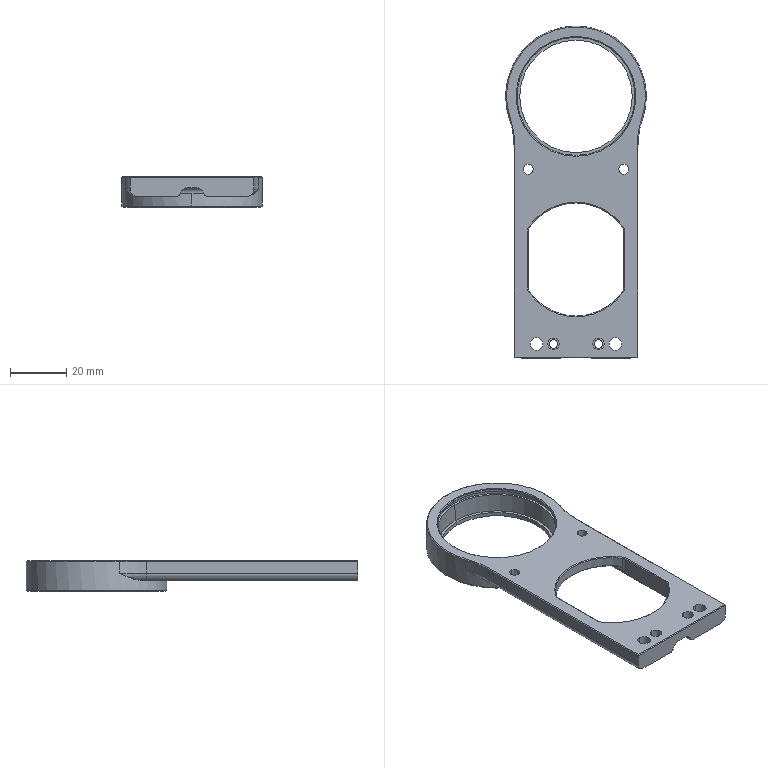NC program | NX | posted with a generic post | part box 50 x 118 x 11 mm
Lines 19 to 843 of 3723:
(ZLEVEL_PROFILE , TOOL : D10)
N36 T15 M6
N38 G54
N40 G17 G0 G90 X-64.1 Y-13.852 S9500 M3
N42 G43 Z30. H15
N44 Z1.5
N46 G94 G1 Y22.554 Z-0.408 F1000.
N48 X-63.766 Y23.898 Z-0.481
N50 X-63.084 Y25.104 Z-0.553
N52 X-62.104 Y26.084 Z-0.626
N54 X-60.898 Y26.766 Z-0.698
N56 X-59.554 Y27.1 Z-0.771
N58 X-59. Z-0.8
N60 X16.084 F3500.
N62 G3 X24.195 Y28.458 R24.9
N64 G2 X24.195 Y-28.458 R-30.1
N66 G3 X16.084 Y-27.1 R24.9
N68 G1 X-59.
N70 G2 X-64.1 Y-22. R5.1
N72 G1 Y22.
N74 G2 X-59. Y27.1 R5.1
N76 G1 X16.084 Z-0.976
N78 X17.116 Y27.121 Z-0.978
N80 X18.147 Y27.186 Z-0.981
N82 X19.174 Y27.293 Z-0.983
N84 X20.196 Y27.442 Z-0.986
N86 X21.21 Y27.634 Z-0.988
N88 X22.216 Y27.867 Z-0.991
N90 X23.212 Y28.142 Z-0.993
N92 X24.195 Y28.458 Z-0.995
N94 X25.435 Y28.856 Z-0.998
N96 X26.691 Y29.199 Z-1.002
N98 X27.96 Y29.488 Z-1.005
N100 X29.241 Y29.721 Z-1.008
N102 X30.531 Y29.899 Z-1.011
N104 X31.827 Y30.021 Z-1.014
N106 X33.127 Y30.087 Z-1.017
N108 X34.429 Y30.097 Z-1.02
N110 X35.731 Y30.05 Z-1.023
N112 X37.028 Y29.947 Z-1.026
N114 X38.321 Y29.788 Z-1.029
N116 X39.605 Y29.574 Z-1.032
N118 X40.879 Y29.304 Z-1.035
N120 X42.139 Y28.979 Z-1.038
N122 X43.385 Y28.6 Z-1.041
N124 X44.613 Y28.167 Z-1.044
N126 X45.821 Y27.682 Z-1.047
N128 X47.007 Y27.144 Z-1.05
N130 X48.169 Y26.557 Z-1.053
N132 X49.304 Y25.919 Z-1.056
N134 X50.411 Y25.233 Z-1.06
N136 X51.487 Y24.5 Z-1.063
N138 X52.53 Y23.72 Z-1.066
N140 X53.538 Y22.897 Z-1.069
N142 X54.51 Y22.031 Z-1.072
N144 X55.444 Y21.123 Z-1.075
N146 X56.337 Y20.176 Z-1.078
N148 X57.189 Y19.191 Z-1.081
N150 X57.997 Y18.17 Z-1.084
N152 X58.76 Y17.115 Z-1.087
N154 X59.477 Y16.029 Z-1.09
N156 X60.147 Y14.912 Z-1.093
N158 X60.767 Y13.767 Z-1.096
N160 X61.337 Y12.597 Z-1.099
N162 X61.857 Y11.403 Z-1.102
N164 X62.324 Y10.187 Z-1.105
N166 X62.738 Y8.953 Z-1.108
N168 X63.098 Y7.702 Z-1.111
N170 X63.404 Y6.436 Z-1.114
N172 X63.655 Y5.159 Z-1.118
N174 X63.85 Y3.871 Z-1.121
N176 X63.989 Y2.577 Z-1.124
N178 X64.073 Y1.278 Z-1.127
N180 X64.1 Y-0.024 Z-1.13
N182 X64.071 Y-1.325 Z-1.133
N184 X63.986 Y-2.623 Z-1.136
N186 X63.844 Y-3.916 Z-1.139
N188 X63.647 Y-5.202 Z-1.142
N190 X63.395 Y-6.478 Z-1.145
N192 X63.087 Y-7.742 Z-1.148
N194 X62.726 Y-8.992 Z-1.151
N196 X62.31 Y-10.225 Z-1.154
N198 X61.842 Y-11.438 Z-1.157
N200 X61.322 Y-12.631 Z-1.16
N202 X60.75 Y-13.799 Z-1.163
N204 X60.129 Y-14.942 Z-1.166
N206 X59.459 Y-16.057 Z-1.169
N208 X58.742 Y-17.143 Z-1.172
N210 X57.978 Y-18.196 Z-1.175
N212 X57.169 Y-19.215 Z-1.179
N214 X56.317 Y-20.198 Z-1.182
N216 X55.424 Y-21.143 Z-1.185
N218 X54.49 Y-22.049 Z-1.188
N220 X53.518 Y-22.914 Z-1.191
N222 X52.51 Y-23.736 Z-1.194
N224 X51.467 Y-24.514 Z-1.197
N226 X50.391 Y-25.245 Z-1.2
N228 X49.285 Y-25.93 Z-1.203
N230 X48.151 Y-26.566 Z-1.206
N232 X46.989 Y-27.153 Z-1.209
N234 X45.804 Y-27.689 Z-1.212
N236 X44.597 Y-28.173 Z-1.215
N238 X43.369 Y-28.605 Z-1.218
N240 X42.125 Y-28.983 Z-1.221
N242 X40.865 Y-29.307 Z-1.224
N244 X39.592 Y-29.576 Z-1.227
N246 X38.309 Y-29.79 Z-1.23
N248 X37.018 Y-29.948 Z-1.233
N250 X35.721 Y-30.051 Z-1.236
N252 X34.421 Y-30.097 Z-1.24
N254 X33.12 Y-30.087 Z-1.243
N256 X31.82 Y-30.021 Z-1.246
N258 X30.525 Y-29.899 Z-1.249
N260 X29.237 Y-29.721 Z-1.252
N262 X27.957 Y-29.487 Z-1.255
N264 X26.688 Y-29.198 Z-1.258
N266 X25.434 Y-28.855 Z-1.261
N268 X24.195 Y-28.458 Z-1.264
N270 X23.212 Y-28.142 Z-1.266
N272 X22.216 Y-27.867 Z-1.269
N274 X21.21 Y-27.634 Z-1.271
N276 X20.196 Y-27.442 Z-1.274
N278 X19.174 Y-27.293 Z-1.276
N280 X18.147 Y-27.186 Z-1.278
N282 X17.116 Y-27.121 Z-1.281
N284 X16.084 Y-27.1 Z-1.283
N286 X-59. Z-1.459
N288 X-59.5 Y-27.075 Z-1.46
N290 X-59.995 Y-27.002 Z-1.462
N292 X-60.48 Y-26.88 Z-1.463
N294 X-60.952 Y-26.712 Z-1.464
N296 X-61.404 Y-26.498 Z-1.465
N298 X-61.833 Y-26.24 Z-1.466
N300 X-62.235 Y-25.942 Z-1.468
N302 X-62.606 Y-25.606 Z-1.469
N304 X-62.942 Y-25.235 Z-1.47
N306 X-63.24 Y-24.833 Z-1.471
N308 X-63.498 Y-24.404 Z-1.472
N310 X-63.712 Y-23.952 Z-1.473
N312 X-63.88 Y-23.48 Z-1.475
N314 X-64.002 Y-22.995 Z-1.476
N316 X-64.075 Y-22.5 Z-1.477
N318 X-64.1 Y-22. Z-1.478
N320 Y22. Z-1.581
N322 X-64.075 Y22.5 Z-1.582
N324 X-64.002 Y22.995 Z-1.584
N326 X-63.88 Y23.48 Z-1.585
N328 X-63.712 Y23.952 Z-1.586
N330 X-63.498 Y24.404 Z-1.587
N332 X-63.24 Y24.833 Z-1.588
N334 X-62.942 Y25.235 Z-1.589
N336 X-62.606 Y25.606 Z-1.591
N338 X-62.235 Y25.942 Z-1.592
N340 X-61.833 Y26.24 Z-1.593
N342 X-61.404 Y26.498 Z-1.594
N344 X-60.952 Y26.712 Z-1.595
N346 X-60.48 Y26.88 Z-1.596
N348 X-59.995 Y27.002 Z-1.598
N350 X-59.5 Y27.075 Z-1.599
N352 X-59. Y27.1 Z-1.6
N354 X16.084 Z-1.776
N356 X17.116 Y27.121 Z-1.778
N358 X18.147 Y27.186 Z-1.781
N360 X19.174 Y27.293 Z-1.783
N362 X20.196 Y27.442 Z-1.786
N364 X21.21 Y27.634 Z-1.788
N366 X22.216 Y27.867 Z-1.791
N368 X23.212 Y28.142 Z-1.793
N370 X24.195 Y28.458 Z-1.795
N372 X25.435 Y28.856 Z-1.798
N374 X26.691 Y29.199 Z-1.802
N376 X27.96 Y29.488 Z-1.805
N378 X29.241 Y29.721 Z-1.808
N380 X30.531 Y29.899 Z-1.811
N382 X31.827 Y30.021 Z-1.814
N384 X33.127 Y30.087 Z-1.817
N386 X34.429 Y30.097 Z-1.82
N388 X35.731 Y30.05 Z-1.823
N390 X37.028 Y29.947 Z-1.826
N392 X38.321 Y29.788 Z-1.829
N394 X39.605 Y29.574 Z-1.832
N396 X40.879 Y29.304 Z-1.835
N398 X42.139 Y28.979 Z-1.838
N400 X43.385 Y28.6 Z-1.841
N402 X44.613 Y28.167 Z-1.844
N404 X45.821 Y27.682 Z-1.847
N406 X47.007 Y27.144 Z-1.85
N408 X48.169 Y26.557 Z-1.853
N410 X49.304 Y25.919 Z-1.856
N412 X50.411 Y25.233 Z-1.86
N414 X51.487 Y24.5 Z-1.863
N416 X52.53 Y23.72 Z-1.866
N418 X53.538 Y22.897 Z-1.869
N420 X54.51 Y22.031 Z-1.872
N422 X55.444 Y21.123 Z-1.875
N424 X56.337 Y20.176 Z-1.878
N426 X57.189 Y19.191 Z-1.881
N428 X57.997 Y18.17 Z-1.884
N430 X58.76 Y17.115 Z-1.887
N432 X59.477 Y16.029 Z-1.89
N434 X60.147 Y14.912 Z-1.893
N436 X60.767 Y13.767 Z-1.896
N438 X61.337 Y12.597 Z-1.899
N440 X61.857 Y11.403 Z-1.902
N442 X62.324 Y10.187 Z-1.905
N444 X62.738 Y8.953 Z-1.908
N446 X63.098 Y7.702 Z-1.911
N448 X63.404 Y6.436 Z-1.914
N450 X63.655 Y5.159 Z-1.918
N452 X63.85 Y3.871 Z-1.921
N454 X63.989 Y2.577 Z-1.924
N456 X64.073 Y1.278 Z-1.927
N458 X64.1 Y-0.024 Z-1.93
N460 X64.071 Y-1.325 Z-1.933
N462 X63.986 Y-2.623 Z-1.936
N464 X63.844 Y-3.916 Z-1.939
N466 X63.647 Y-5.202 Z-1.942
N468 X63.395 Y-6.478 Z-1.945
N470 X63.087 Y-7.742 Z-1.948
N472 X62.726 Y-8.992 Z-1.951
N474 X62.31 Y-10.225 Z-1.954
N476 X61.842 Y-11.438 Z-1.957
N478 X61.322 Y-12.631 Z-1.96
N480 X60.75 Y-13.799 Z-1.963
N482 X60.129 Y-14.942 Z-1.966
N484 X59.459 Y-16.057 Z-1.969
N486 X58.742 Y-17.143 Z-1.972
N488 X57.978 Y-18.196 Z-1.975
N490 X57.169 Y-19.215 Z-1.979
N492 X56.317 Y-20.198 Z-1.982
N494 X55.424 Y-21.143 Z-1.985
N496 X54.49 Y-22.049 Z-1.988
N498 X53.518 Y-22.914 Z-1.991
N500 X52.51 Y-23.736 Z-1.994
N502 X51.467 Y-24.514 Z-1.997
N504 X50.391 Y-25.245 Z-2.
N506 X49.285 Y-25.93 Z-2.003
N508 X48.151 Y-26.566 Z-2.006
N510 X46.989 Y-27.153 Z-2.009
N512 X45.804 Y-27.689 Z-2.012
N514 X44.597 Y-28.173 Z-2.015
N516 X43.369 Y-28.605 Z-2.018
N518 X42.125 Y-28.983 Z-2.021
N520 X40.865 Y-29.307 Z-2.024
N522 X39.592 Y-29.576 Z-2.027
N524 X38.309 Y-29.79 Z-2.03
N526 X37.018 Y-29.948 Z-2.033
N528 X35.721 Y-30.051 Z-2.036
N530 X34.421 Y-30.097 Z-2.04
N532 X33.12 Y-30.087 Z-2.043
N534 X31.82 Y-30.021 Z-2.046
N536 X30.525 Y-29.899 Z-2.049
N538 X29.237 Y-29.721 Z-2.052
N540 X27.957 Y-29.487 Z-2.055
N542 X26.688 Y-29.198 Z-2.058
N544 X25.434 Y-28.855 Z-2.061
N546 X24.195 Y-28.458 Z-2.064
N548 X23.212 Y-28.142 Z-2.066
N550 X22.216 Y-27.867 Z-2.069
N552 X21.21 Y-27.634 Z-2.071
N554 X20.196 Y-27.442 Z-2.074
N556 X19.174 Y-27.293 Z-2.076
N558 X18.147 Y-27.186 Z-2.078
N560 X17.116 Y-27.121 Z-2.081
N562 X16.084 Y-27.1 Z-2.083
N564 X-59. Z-2.259
N566 X-59.5 Y-27.075 Z-2.26
N568 X-59.995 Y-27.002 Z-2.262
N570 X-60.48 Y-26.88 Z-2.263
N572 X-60.952 Y-26.712 Z-2.264
N574 X-61.404 Y-26.498 Z-2.265
N576 X-61.833 Y-26.24 Z-2.266
N578 X-62.235 Y-25.942 Z-2.268
N580 X-62.606 Y-25.606 Z-2.269
N582 X-62.942 Y-25.235 Z-2.27
N584 X-63.24 Y-24.833 Z-2.271
N586 X-63.498 Y-24.404 Z-2.272
N588 X-63.712 Y-23.952 Z-2.273
N590 X-63.88 Y-23.48 Z-2.275
N592 X-64.002 Y-22.995 Z-2.276
N594 X-64.075 Y-22.5 Z-2.277
N596 X-64.1 Y-22. Z-2.278
N598 Y22. Z-2.381
N600 X-64.075 Y22.5 Z-2.382
N602 X-64.002 Y22.995 Z-2.384
N604 X-63.88 Y23.48 Z-2.385
N606 X-63.712 Y23.952 Z-2.386
N608 X-63.498 Y24.404 Z-2.387
N610 X-63.24 Y24.833 Z-2.388
N612 X-62.942 Y25.235 Z-2.389
N614 X-62.606 Y25.606 Z-2.391
N616 X-62.235 Y25.942 Z-2.392
N618 X-61.833 Y26.24 Z-2.393
N620 X-61.404 Y26.498 Z-2.394
N622 X-60.952 Y26.712 Z-2.395
N624 X-60.48 Y26.88 Z-2.396
N626 X-59.995 Y27.002 Z-2.398
N628 X-59.5 Y27.075 Z-2.399
N630 X-59. Y27.1 Z-2.4
N632 X16.084 Z-2.583
N634 X17.116 Y27.121 Z-2.586
N636 X18.147 Y27.186 Z-2.588
N638 X19.174 Y27.293 Z-2.591
N640 X20.196 Y27.442 Z-2.593
N642 X21.21 Y27.634 Z-2.596
N644 X22.216 Y27.867 Z-2.599
N646 X23.212 Y28.142 Z-2.601
N648 X24.195 Y28.458 Z-2.604
N650 X25.435 Y28.856 Z-2.607
N652 X26.691 Y29.199 Z-2.61
N654 X27.96 Y29.488 Z-2.613
N656 X29.241 Y29.721 Z-2.616
N658 X30.531 Y29.899 Z-2.619
N660 X31.827 Y30.021 Z-2.623
N662 X33.127 Y30.087 Z-2.626
N664 X34.429 Y30.097 Z-2.629
N666 X35.731 Y30.05 Z-2.632
N668 X37.028 Y29.947 Z-2.635
N670 X38.321 Y29.788 Z-2.639
N672 X39.605 Y29.574 Z-2.642
N674 X40.879 Y29.304 Z-2.645
N676 X42.139 Y28.979 Z-2.648
N678 X43.385 Y28.6 Z-2.651
N680 X44.613 Y28.167 Z-2.654
N682 X45.821 Y27.682 Z-2.658
N684 X47.007 Y27.144 Z-2.661
N686 X48.169 Y26.557 Z-2.664
N688 X49.304 Y25.919 Z-2.667
N690 X50.411 Y25.233 Z-2.67
N692 X51.487 Y24.5 Z-2.674
N694 X52.53 Y23.72 Z-2.677
N696 X53.538 Y22.897 Z-2.68
N698 X54.51 Y22.031 Z-2.683
N700 X55.444 Y21.123 Z-2.686
N702 X56.337 Y20.176 Z-2.689
N704 X57.189 Y19.191 Z-2.693
N706 X57.997 Y18.17 Z-2.696
N708 X58.76 Y17.115 Z-2.699
N710 X59.477 Y16.029 Z-2.702
N712 X60.147 Y14.912 Z-2.705
N714 X60.767 Y13.767 Z-2.708
N716 X61.337 Y12.597 Z-2.712
N718 X61.857 Y11.403 Z-2.715
N720 X62.324 Y10.187 Z-2.718
N722 X62.738 Y8.953 Z-2.721
N724 X63.098 Y7.702 Z-2.724
N726 X63.404 Y6.436 Z-2.728
N728 X63.655 Y5.159 Z-2.731
N730 X63.85 Y3.871 Z-2.734
N732 X63.989 Y2.577 Z-2.737
N734 X64.073 Y1.278 Z-2.74
N736 X64.1 Y-0.024 Z-2.743
N738 X64.071 Y-1.325 Z-2.747
N740 X63.986 Y-2.623 Z-2.75
N742 X63.844 Y-3.916 Z-2.753
N744 X63.647 Y-5.202 Z-2.756
N746 X63.395 Y-6.478 Z-2.759
N748 X63.087 Y-7.742 Z-2.763
N750 X62.726 Y-8.992 Z-2.766
N752 X62.31 Y-10.225 Z-2.769
N754 X61.842 Y-11.438 Z-2.772
N756 X61.322 Y-12.631 Z-2.775
N758 X60.75 Y-13.799 Z-2.778
N760 X60.129 Y-14.942 Z-2.782
N762 X59.459 Y-16.057 Z-2.785
N764 X58.742 Y-17.143 Z-2.788
N766 X57.978 Y-18.196 Z-2.791
N768 X57.169 Y-19.215 Z-2.794
N770 X56.317 Y-20.198 Z-2.797
N772 X55.424 Y-21.143 Z-2.801
N774 X54.49 Y-22.049 Z-2.804
N776 X53.518 Y-22.914 Z-2.807
N778 X52.51 Y-23.736 Z-2.81
N780 X51.467 Y-24.514 Z-2.813
N782 X50.391 Y-25.245 Z-2.817
N784 X49.285 Y-25.93 Z-2.82
N786 X48.151 Y-26.566 Z-2.823
N788 X46.989 Y-27.153 Z-2.826
N790 X45.804 Y-27.689 Z-2.829
N792 X44.597 Y-28.173 Z-2.832
N794 X43.369 Y-28.605 Z-2.836
N796 X42.125 Y-28.983 Z-2.839
N798 X40.865 Y-29.307 Z-2.842
N800 X39.592 Y-29.576 Z-2.845
N802 X38.309 Y-29.79 Z-2.848
N804 X37.018 Y-29.948 Z-2.851
N806 X35.721 Y-30.051 Z-2.855
N808 X34.421 Y-30.097 Z-2.858
N810 X33.12 Y-30.087 Z-2.861
N812 X31.82 Y-30.021 Z-2.864
N814 X30.525 Y-29.899 Z-2.867
N816 X29.237 Y-29.721 Z-2.871
N818 X27.957 Y-29.487 Z-2.874
N820 X26.688 Y-29.198 Z-2.877
N822 X25.434 Y-28.855 Z-2.88
N824 X24.195 Y-28.458 Z-2.883
N826 X23.212 Y-28.142 Z-2.886
N828 X22.216 Y-27.867 Z-2.888
N830 X21.21 Y-27.634 Z-2.891
N832 X20.196 Y-27.442 Z-2.893
N834 X19.174 Y-27.293 Z-2.896
N836 X18.147 Y-27.186 Z-2.898
N838 X17.116 Y-27.121 Z-2.901
N840 X16.084 Y-27.1 Z-2.903
N842 X-59. Z-3.087
N844 X-59.5 Y-27.075 Z-3.088
N846 X-59.995 Y-27.002 Z-3.089
N848 X-60.48 Y-26.88 Z-3.09
N850 X-60.952 Y-26.712 Z-3.092
N852 X-61.404 Y-26.498 Z-3.093
N854 X-61.833 Y-26.24 Z-3.094
N856 X-62.235 Y-25.942 Z-3.095
N858 X-62.606 Y-25.606 Z-3.097
N860 X-62.942 Y-25.235 Z-3.098
N862 X-63.24 Y-24.833 Z-3.099
N864 X-63.498 Y-24.404 Z-3.1
N866 X-63.712 Y-23.952 Z-3.101
N868 X-63.88 Y-23.48 Z-3.103
N870 X-64.002 Y-22.995 Z-3.104
N872 X-64.075 Y-22.5 Z-3.105
N874 X-64.1 Y-22. Z-3.106
N876 Y22. Z-3.214
N878 X-64.075 Y22.5 Z-3.215
N880 X-64.002 Y22.995 Z-3.216
N882 X-63.88 Y23.48 Z-3.217
N884 X-63.712 Y23.952 Z-3.219
N886 X-63.498 Y24.404 Z-3.22
N888 X-63.24 Y24.833 Z-3.221
N890 X-62.942 Y25.235 Z-3.222
N892 X-62.606 Y25.606 Z-3.224
N894 X-62.235 Y25.942 Z-3.225
N896 X-61.833 Y26.24 Z-3.226
N898 X-61.404 Y26.498 Z-3.227
N900 X-60.952 Y26.712 Z-3.228
N902 X-60.48 Y26.88 Z-3.23
N904 X-59.995 Y27.002 Z-3.231
N906 X-59.5 Y27.075 Z-3.232
N908 X-59. Y27.1 Z-3.233
N910 X16.084 Z-3.417
N912 X17.116 Y27.121 Z-3.419
N914 X18.147 Y27.186 Z-3.422
N916 X19.174 Y27.293 Z-3.424
N918 X20.196 Y27.442 Z-3.427
N920 X21.21 Y27.634 Z-3.429
N922 X22.216 Y27.867 Z-3.432
N924 X23.212 Y28.142 Z-3.434
N926 X24.195 Y28.458 Z-3.437
N928 X25.435 Y28.856 Z-3.44
N930 X26.691 Y29.199 Z-3.443
N932 X27.96 Y29.488 Z-3.446
N934 X29.241 Y29.721 Z-3.45
N936 X30.531 Y29.899 Z-3.453
N938 X31.827 Y30.021 Z-3.456
N940 X33.127 Y30.087 Z-3.459
N942 X34.429 Y30.097 Z-3.462
N944 X35.731 Y30.05 Z-3.466
N946 X37.028 Y29.947 Z-3.469
N948 X38.321 Y29.788 Z-3.472
N950 X39.605 Y29.574 Z-3.475
N952 X40.879 Y29.304 Z-3.478
N954 X42.139 Y28.979 Z-3.481
N956 X43.385 Y28.6 Z-3.485
N958 X44.613 Y28.167 Z-3.488
N960 X45.821 Y27.682 Z-3.491
N962 X47.007 Y27.144 Z-3.494
N964 X48.169 Y26.557 Z-3.497
N966 X49.304 Y25.919 Z-3.5
N968 X50.411 Y25.233 Z-3.504
N970 X51.487 Y24.5 Z-3.507
N972 X52.53 Y23.72 Z-3.51
N974 X53.538 Y22.897 Z-3.513
N976 X54.51 Y22.031 Z-3.516
N978 X55.444 Y21.123 Z-3.52
N980 X56.337 Y20.176 Z-3.523
N982 X57.189 Y19.191 Z-3.526
N984 X57.997 Y18.17 Z-3.529
N986 X58.76 Y17.115 Z-3.532
N988 X59.477 Y16.029 Z-3.535
N990 X60.147 Y14.912 Z-3.539
N992 X60.767 Y13.767 Z-3.542
N994 X61.337 Y12.597 Z-3.545
N996 X61.857 Y11.403 Z-3.548
N998 X62.324 Y10.187 Z-3.551
N1000 X62.738 Y8.953 Z-3.555
N1002 X63.098 Y7.702 Z-3.558
N1004 X63.404 Y6.436 Z-3.561
N1006 X63.655 Y5.159 Z-3.564
N1008 X63.85 Y3.871 Z-3.567
N1010 X63.989 Y2.577 Z-3.57
N1012 X64.073 Y1.278 Z-3.574
N1014 X64.1 Y-0.024 Z-3.577
N1016 X64.071 Y-1.325 Z-3.58
N1018 X63.986 Y-2.623 Z-3.583
N1020 X63.844 Y-3.916 Z-3.586
N1022 X63.647 Y-5.202 Z-3.589
N1024 X63.395 Y-6.478 Z-3.593
N1026 X63.087 Y-7.742 Z-3.596
N1028 X62.726 Y-8.992 Z-3.599
N1030 X62.31 Y-10.225 Z-3.602
N1032 X61.842 Y-11.438 Z-3.605
N1034 X61.322 Y-12.631 Z-3.609
N1036 X60.75 Y-13.799 Z-3.612
N1038 X60.129 Y-14.942 Z-3.615
N1040 X59.459 Y-16.057 Z-3.618
N1042 X58.742 Y-17.143 Z-3.621
N1044 X57.978 Y-18.196 Z-3.624
N1046 X57.169 Y-19.215 Z-3.628
N1048 X56.317 Y-20.198 Z-3.631
N1050 X55.424 Y-21.143 Z-3.634
N1052 X54.49 Y-22.049 Z-3.637
N1054 X53.518 Y-22.914 Z-3.64
N1056 X52.51 Y-23.736 Z-3.644
N1058 X51.467 Y-24.514 Z-3.647
N1060 X50.391 Y-25.245 Z-3.65
N1062 X49.285 Y-25.93 Z-3.653
N1064 X48.151 Y-26.566 Z-3.656
N1066 X46.989 Y-27.153 Z-3.659
N1068 X45.804 Y-27.689 Z-3.663
N1070 X44.597 Y-28.173 Z-3.666
N1072 X43.369 Y-28.605 Z-3.669
N1074 X42.125 Y-28.983 Z-3.672
N1076 X40.865 Y-29.307 Z-3.675
N1078 X39.592 Y-29.576 Z-3.678
N1080 X38.309 Y-29.79 Z-3.682
N1082 X37.018 Y-29.948 Z-3.685
N1084 X35.721 Y-30.051 Z-3.688
N1086 X34.421 Y-30.097 Z-3.691
N1088 X33.12 Y-30.087 Z-3.694
N1090 X31.82 Y-30.021 Z-3.698
N1092 X30.525 Y-29.899 Z-3.701
N1094 X29.237 Y-29.721 Z-3.704
N1096 X27.957 Y-29.487 Z-3.707
N1098 X26.688 Y-29.198 Z-3.71
N1100 X25.434 Y-28.855 Z-3.713
N1102 X24.195 Y-28.458 Z-3.717
N1104 X23.212 Y-28.142 Z-3.719
N1106 X22.216 Y-27.867 Z-3.722
N1108 X21.21 Y-27.634 Z-3.724
N1110 X20.196 Y-27.442 Z-3.727
N1112 X19.174 Y-27.293 Z-3.729
N1114 X18.147 Y-27.186 Z-3.732
N1116 X17.116 Y-27.121 Z-3.734
N1118 X16.084 Y-27.1 Z-3.737
N1120 X-59. Z-3.92
N1122 X-59.5 Y-27.075 Z-3.921
N1124 X-59.995 Y-27.002 Z-3.923
N1126 X-60.48 Y-26.88 Z-3.924
N1128 X-60.952 Y-26.712 Z-3.925
N1130 X-61.404 Y-26.498 Z-3.926
N1132 X-61.833 Y-26.24 Z-3.927
N1134 X-62.235 Y-25.942 Z-3.929
N1136 X-62.606 Y-25.606 Z-3.93
N1138 X-62.942 Y-25.235 Z-3.931
N1140 X-63.24 Y-24.833 Z-3.932
N1142 X-63.498 Y-24.404 Z-3.934
N1144 X-63.712 Y-23.952 Z-3.935
N1146 X-63.88 Y-23.48 Z-3.936
N1148 X-64.002 Y-22.995 Z-3.937
N1150 X-64.075 Y-22.5 Z-3.938
N1152 X-64.1 Y-22. Z-3.94
N1154 Y22. Z-4.047
N1156 X-64.075 Y22.5 Z-4.048
N1158 X-64.002 Y22.995 Z-4.05
N1160 X-63.88 Y23.48 Z-4.051
N1162 X-63.712 Y23.952 Z-4.052
N1164 X-63.498 Y24.404 Z-4.053
N1166 X-63.24 Y24.833 Z-4.054
N1168 X-62.942 Y25.235 Z-4.056
N1170 X-62.606 Y25.606 Z-4.057
N1172 X-62.235 Y25.942 Z-4.058
N1174 X-61.833 Y26.24 Z-4.059
N1176 X-61.404 Y26.498 Z-4.061
N1178 X-60.952 Y26.712 Z-4.062
N1180 X-60.48 Y26.88 Z-4.063
N1182 X-59.995 Y27.002 Z-4.064
N1184 X-59.5 Y27.075 Z-4.065
N1186 X-59. Y27.1 Z-4.067
N1188 X16.084 Z-4.25
N1190 X17.116 Y27.121 Z-4.253
N1192 X18.147 Y27.186 Z-4.255
N1194 X19.174 Y27.293 Z-4.258
N1196 X20.196 Y27.442 Z-4.26
N1198 X21.21 Y27.634 Z-4.263
N1200 X22.216 Y27.867 Z-4.265
N1202 X23.212 Y28.142 Z-4.268
N1204 X24.195 Y28.458 Z-4.27
N1206 X25.435 Y28.856 Z-4.273
N1208 X26.691 Y29.199 Z-4.277
N1210 X27.96 Y29.488 Z-4.28
N1212 X29.241 Y29.721 Z-4.283
N1214 X30.531 Y29.899 Z-4.286
N1216 X31.827 Y30.021 Z-4.289
N1218 X33.127 Y30.087 Z-4.292
N1220 X34.429 Y30.097 Z-4.296
N1222 X35.731 Y30.05 Z-4.299
N1224 X37.028 Y29.947 Z-4.302
N1226 X38.321 Y29.788 Z-4.305
N1228 X39.605 Y29.574 Z-4.308
N1230 X40.879 Y29.304 Z-4.312
N1232 X42.139 Y28.979 Z-4.315
N1234 X43.385 Y28.6 Z-4.318
N1236 X44.613 Y28.167 Z-4.321
N1238 X45.821 Y27.682 Z-4.324
N1240 X47.007 Y27.144 Z-4.327
N1242 X48.169 Y26.557 Z-4.331
N1244 X49.304 Y25.919 Z-4.334
N1246 X50.411 Y25.233 Z-4.337
N1248 X51.487 Y24.5 Z-4.34
N1250 X52.53 Y23.72 Z-4.343
N1252 X53.538 Y22.897 Z-4.347
N1254 X54.51 Y22.031 Z-4.35
N1256 X55.444 Y21.123 Z-4.353
N1258 X56.337 Y20.176 Z-4.356
N1260 X57.189 Y19.191 Z-4.359
N1262 X57.997 Y18.17 Z-4.362
N1264 X58.76 Y17.115 Z-4.366
N1266 X59.477 Y16.029 Z-4.369
N1268 X60.147 Y14.912 Z-4.372
N1270 X60.767 Y13.767 Z-4.375
N1272 X61.337 Y12.597 Z-4.378
N1274 X61.857 Y11.403 Z-4.382
N1276 X62.324 Y10.187 Z-4.385
N1278 X62.738 Y8.953 Z-4.388
N1280 X63.098 Y7.702 Z-4.391
N1282 X63.404 Y6.436 Z-4.394
N1284 X63.655 Y5.159 Z-4.397
N1286 X63.85 Y3.871 Z-4.401
N1288 X63.989 Y2.577 Z-4.404
N1290 X64.073 Y1.278 Z-4.407
N1292 X64.1 Y-0.024 Z-4.41
N1294 X64.071 Y-1.325 Z-4.413
N1296 X63.986 Y-2.623 Z-4.416
N1298 X63.844 Y-3.916 Z-4.42
N1300 X63.647 Y-5.202 Z-4.423
N1302 X63.395 Y-6.478 Z-4.426
N1304 X63.087 Y-7.742 Z-4.429
N1306 X62.726 Y-8.992 Z-4.432
N1308 X62.31 Y-10.225 Z-4.436
N1310 X61.842 Y-11.438 Z-4.439
N1312 X61.322 Y-12.631 Z-4.442
N1314 X60.75 Y-13.799 Z-4.445
N1316 X60.129 Y-14.942 Z-4.448
N1318 X59.459 Y-16.057 Z-4.451
N1320 X58.742 Y-17.143 Z-4.455
N1322 X57.978 Y-18.196 Z-4.458
N1324 X57.169 Y-19.215 Z-4.461
N1326 X56.317 Y-20.198 Z-4.464
N1328 X55.424 Y-21.143 Z-4.467
N1330 X54.49 Y-22.049 Z-4.47
N1332 X53.518 Y-22.914 Z-4.474
N1334 X52.51 Y-23.736 Z-4.477
N1336 X51.467 Y-24.514 Z-4.48
N1338 X50.391 Y-25.245 Z-4.483
N1340 X49.285 Y-25.93 Z-4.486
N1342 X48.151 Y-26.566 Z-4.49
N1344 X46.989 Y-27.153 Z-4.493
N1346 X45.804 Y-27.689 Z-4.496
N1348 X44.597 Y-28.173 Z-4.499
N1350 X43.369 Y-28.605 Z-4.502
N1352 X42.125 Y-28.983 Z-4.505
N1354 X40.865 Y-29.307 Z-4.509
N1356 X39.592 Y-29.576 Z-4.512
N1358 X38.309 Y-29.79 Z-4.515
N1360 X37.018 Y-29.948 Z-4.518
N1362 X35.721 Y-30.051 Z-4.521
N1364 X34.421 Y-30.097 Z-4.524
N1366 X33.12 Y-30.087 Z-4.528
N1368 X31.82 Y-30.021 Z-4.531
N1370 X30.525 Y-29.899 Z-4.534
N1372 X29.237 Y-29.721 Z-4.537
N1374 X27.957 Y-29.487 Z-4.54
N1376 X26.688 Y-29.198 Z-4.544
N1378 X25.434 Y-28.855 Z-4.547
N1380 X24.195 Y-28.458 Z-4.55
N1382 X23.212 Y-28.142 Z-4.552
N1384 X22.216 Y-27.867 Z-4.555
N1386 X21.21 Y-27.634 Z-4.557
N1388 X20.196 Y-27.442 Z-4.56
N1390 X19.174 Y-27.293 Z-4.563
N1392 X18.147 Y-27.186 Z-4.565
N1394 X17.116 Y-27.121 Z-4.568
N1396 X16.084 Y-27.1 Z-4.57
N1398 X-59. Z-4.753
N1400 X-59.5 Y-27.075 Z-4.755
N1402 X-59.995 Y-27.002 Z-4.756
N1404 X-60.48 Y-26.88 Z-4.757
N1406 X-60.952 Y-26.712 Z-4.758
N1408 X-61.404 Y-26.498 Z-4.76
N1410 X-61.833 Y-26.24 Z-4.761
N1412 X-62.235 Y-25.942 Z-4.762
N1414 X-62.606 Y-25.606 Z-4.763
N1416 X-62.942 Y-25.235 Z-4.764
N1418 X-63.24 Y-24.833 Z-4.766
N1420 X-63.498 Y-24.404 Z-4.767
N1422 X-63.712 Y-23.952 Z-4.768
N1424 X-63.88 Y-23.48 Z-4.769
N1426 X-64.002 Y-22.995 Z-4.771
N1428 X-64.075 Y-22.5 Z-4.772
N1430 X-64.1 Y-22. Z-4.773
N1432 Y22. Z-4.88
N1434 X-64.075 Y22.5 Z-4.882
N1436 X-64.002 Y22.995 Z-4.883
N1438 X-63.88 Y23.48 Z-4.884
N1440 X-63.712 Y23.952 Z-4.885
N1442 X-63.498 Y24.404 Z-4.887
N1444 X-63.24 Y24.833 Z-4.888
N1446 X-62.942 Y25.235 Z-4.889
N1448 X-62.606 Y25.606 Z-4.89
N1450 X-62.235 Y25.942 Z-4.891
N1452 X-61.833 Y26.24 Z-4.893
N1454 X-61.404 Y26.498 Z-4.894
N1456 X-60.952 Y26.712 Z-4.895
N1458 X-60.48 Y26.88 Z-4.896
N1460 X-59.995 Y27.002 Z-4.898
N1462 X-59.5 Y27.075 Z-4.899
N1464 X-59. Y27.1 Z-4.9
N1466 X16.084 Z-5.099
N1468 X17.116 Y27.121 Z-5.102
N1470 X18.147 Y27.186 Z-5.105
N1472 X19.174 Y27.293 Z-5.107
N1474 X20.196 Y27.442 Z-5.11
N1476 X21.21 Y27.634 Z-5.113
N1478 X22.216 Y27.867 Z-5.116
N1480 X23.212 Y28.142 Z-5.118
N1482 X24.195 Y28.458 Z-5.121
N1484 X25.435 Y28.856 Z-5.125
N1486 X26.691 Y29.199 Z-5.128
N1488 X27.96 Y29.488 Z-5.131
N1490 X29.241 Y29.721 Z-5.135
N1492 X30.531 Y29.899 Z-5.138
N1494 X31.827 Y30.021 Z-5.142
N1496 X33.127 Y30.087 Z-5.145
N1498 X34.429 Y30.097 Z-5.149
N1500 X35.731 Y30.05 Z-5.152
N1502 X37.028 Y29.947 Z-5.156
N1504 X38.321 Y29.788 Z-5.159
N1506 X39.605 Y29.574 Z-5.163
N1508 X40.879 Y29.304 Z-5.166
N1510 X42.139 Y28.979 Z-5.169
N1512 X43.385 Y28.6 Z-5.173
N1514 X44.613 Y28.167 Z-5.176
N1516 X45.821 Y27.682 Z-5.18
N1518 X47.007 Y27.144 Z-5.183
N1520 X48.169 Y26.557 Z-5.187
N1522 X49.304 Y25.919 Z-5.19
N1524 X50.411 Y25.233 Z-5.194
N1526 X51.487 Y24.5 Z-5.197
N1528 X52.53 Y23.72 Z-5.2
N1530 X53.538 Y22.897 Z-5.204
N1532 X54.51 Y22.031 Z-5.207
N1534 X55.444 Y21.123 Z-5.211
N1536 X56.337 Y20.176 Z-5.214
N1538 X57.189 Y19.191 Z-5.218
N1540 X57.997 Y18.17 Z-5.221
N1542 X58.76 Y17.115 Z-5.225
N1544 X59.477 Y16.029 Z-5.228
N1546 X60.147 Y14.912 Z-5.232
N1548 X60.767 Y13.767 Z-5.235
N1550 X61.337 Y12.597 Z-5.238
N1552 X61.857 Y11.403 Z-5.242
N1554 X62.324 Y10.187 Z-5.245
N1556 X62.738 Y8.953 Z-5.249
N1558 X63.098 Y7.702 Z-5.252
N1560 X63.404 Y6.436 Z-5.256
N1562 X63.655 Y5.159 Z-5.259
N1564 X63.85 Y3.871 Z-5.263
N1566 X63.989 Y2.577 Z-5.266
N1568 X64.073 Y1.278 Z-5.27
N1570 X64.1 Y-0.024 Z-5.273
N1572 X64.071 Y-1.325 Z-5.276
N1574 X63.986 Y-2.623 Z-5.28
N1576 X63.844 Y-3.916 Z-5.283
N1578 X63.647 Y-5.202 Z-5.287
N1580 X63.395 Y-6.478 Z-5.29
N1582 X63.087 Y-7.742 Z-5.294
N1584 X62.726 Y-8.992 Z-5.297
N1586 X62.31 Y-10.225 Z-5.301
N1588 X61.842 Y-11.438 Z-5.304
N1590 X61.322 Y-12.631 Z-5.307
N1592 X60.75 Y-13.799 Z-5.311
N1594 X60.129 Y-14.942 Z-5.314
N1596 X59.459 Y-16.057 Z-5.318
N1598 X58.742 Y-17.143 Z-5.321
N1600 X57.978 Y-18.196 Z-5.325
N1602 X57.169 Y-19.215 Z-5.328
N1604 X56.317 Y-20.198 Z-5.332
N1606 X55.424 Y-21.143 Z-5.335
N1608 X54.49 Y-22.049 Z-5.339
N1610 X53.518 Y-22.914 Z-5.342
N1612 X52.51 Y-23.736 Z-5.345
N1614 X51.467 Y-24.514 Z-5.349
N1616 X50.391 Y-25.245 Z-5.352
N1618 X49.285 Y-25.93 Z-5.356
N1620 X48.151 Y-26.566 Z-5.359
N1622 X46.989 Y-27.153 Z-5.363
N1624 X45.804 Y-27.689 Z-5.366
N1626 X44.597 Y-28.173 Z-5.37
N1628 X43.369 Y-28.605 Z-5.373
N1630 X42.125 Y-28.983 Z-5.376
N1632 X40.865 Y-29.307 Z-5.38
N1634 X39.592 Y-29.576 Z-5.383
N1636 X38.309 Y-29.79 Z-5.387
N1638 X37.018 Y-29.948 Z-5.39
N1640 X35.721 Y-30.051 Z-5.394
N1642 X34.421 Y-30.097 Z-5.397
N1644 X33.12 Y-30.087 Z-5.401
N1646 X31.82 Y-30.021 Z-5.404
N1648 X30.525 Y-29.899 Z-5.408
N1650 X29.237 Y-29.721 Z-5.411
N1652 X27.957 Y-29.487 Z-5.414
N1654 X26.688 Y-29.198 Z-5.418
N1656 X25.434 Y-28.855 Z-5.421
N1658 X24.195 Y-28.458 Z-5.425
N1660 X23.212 Y-28.142 Z-5.428
N1662 X22.216 Y-27.867 Z-5.43
N1664 X21.21 Y-27.634 Z-5.433
N1666 X20.196 Y-27.442 Z-5.436
N1668 X19.174 Y-27.293 Z-5.438
N1670 X18.147 Y-27.186 Z-5.441
N1672 X17.116 Y-27.121 Z-5.444
N1674 X16.084 Y-27.1 Z-5.447
N1676 X-59. Z-5.646
N1678 X-59.5 Y-27.075 Z-5.647